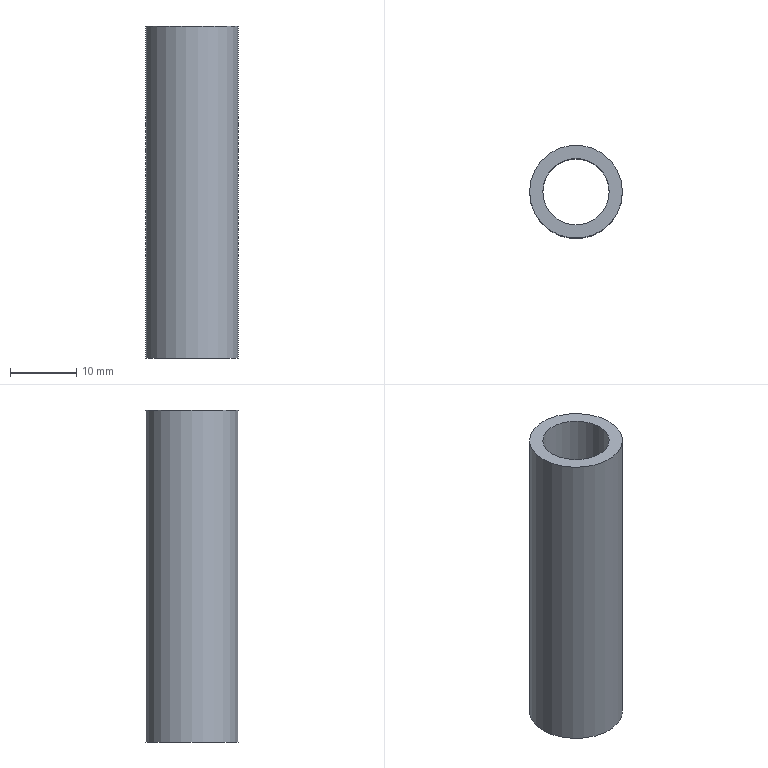Part | NX | features solid 2 | 1 solid | 4 faces | box 14 x 14 x 50 mm | volume 3770 mm3 | plane 2 | cylinder 2 | commonest cylinder face diameters 10 x1 14 x1
STEP:
#1=CARTESIAN_POINT('',(-1253.358,278.112,0.));
#2=VERTEX_POINT('',#1);
#3=CARTESIAN_POINT('',(-1258.358,278.112,0.));
#4=DIRECTION('',(0.,0.,1.));
#5=DIRECTION('',(1.,0.,0.));
#6=AXIS2_PLACEMENT_3D('',#3,#4,#5);
#7=CIRCLE('',#6,5.);
#8=EDGE_CURVE('',#2,#2,#7,.F.);
#9=ORIENTED_EDGE('',*,*,#8,.T.);
#10=EDGE_LOOP('',(#9));
#11=FACE_BOUND('',#10,.T.);
#12=CARTESIAN_POINT('',(-1265.358,278.112,0.));
#13=VERTEX_POINT('',#12);
#14=CARTESIAN_POINT('',(-1258.358,278.112,0.));
#15=DIRECTION('',(0.,0.,-1.));
#16=DIRECTION('',(-1.,0.,0.));
#17=AXIS2_PLACEMENT_3D('',#14,#15,#16);
#18=CIRCLE('',#17,7.);
#19=EDGE_CURVE('',#13,#13,#18,.T.);
#20=ORIENTED_EDGE('',*,*,#19,.F.);
#21=EDGE_LOOP('',(#20));
#22=FACE_BOUND('',#21,.T.);
#23=CARTESIAN_POINT('',(-1258.358,278.112,0.));
#24=DIRECTION('',(0.,0.,1.));
#25=DIRECTION('',(1.,0.,0.));
#26=AXIS2_PLACEMENT_3D('',#23,#24,#25);
#27=PLANE('',#26);
#28=ADVANCED_FACE('',(#11,#22),#27,.T.);
#29=CARTESIAN_POINT('',(-1253.358,278.112,-50.));
#30=VERTEX_POINT('',#29);
#31=CARTESIAN_POINT('',(-1258.358,278.112,-50.));
#32=DIRECTION('',(0.,0.,1.));
#33=DIRECTION('',(1.,0.,0.));
#34=AXIS2_PLACEMENT_3D('',#31,#32,#33);
#35=CIRCLE('',#34,5.);
#36=EDGE_CURVE('',#30,#30,#35,.F.);
#37=ORIENTED_EDGE('',*,*,#36,.F.);
#38=EDGE_LOOP('',(#37));
#39=FACE_BOUND('',#38,.T.);
#40=CARTESIAN_POINT('',(-1265.358,278.112,-50.));
#41=VERTEX_POINT('',#40);
#42=CARTESIAN_POINT('',(-1258.358,278.112,-50.));
#43=DIRECTION('',(0.,0.,-1.));
#44=DIRECTION('',(-1.,0.,0.));
#45=AXIS2_PLACEMENT_3D('',#42,#43,#44);
#46=CIRCLE('',#45,7.);
#47=EDGE_CURVE('',#41,#41,#46,.T.);
#48=ORIENTED_EDGE('',*,*,#47,.T.);
#49=EDGE_LOOP('',(#48));
#50=FACE_BOUND('',#49,.T.);
#51=CARTESIAN_POINT('',(-1258.358,278.112,-50.));
#52=DIRECTION('',(0.,0.,1.));
#53=DIRECTION('',(1.,0.,0.));
#54=AXIS2_PLACEMENT_3D('',#51,#52,#53);
#55=PLANE('',#54);
#56=ADVANCED_FACE('',(#39,#50),#55,.F.);
#57=ORIENTED_EDGE('',*,*,#8,.F.);
#58=EDGE_LOOP('',(#57));
#59=FACE_BOUND('',#58,.T.);
#60=ORIENTED_EDGE('',*,*,#36,.T.);
#61=EDGE_LOOP('',(#60));
#62=FACE_BOUND('',#61,.T.);
#63=CARTESIAN_POINT('',(-1258.358,278.112,-50.));
#64=DIRECTION('',(0.,0.,1.));
#65=DIRECTION('',(1.,0.,0.));
#66=AXIS2_PLACEMENT_3D('',#63,#64,#65);
#67=CYLINDRICAL_SURFACE('',#66,5.);
#68=ADVANCED_FACE('',(#59,#62),#67,.F.);
#69=ORIENTED_EDGE('',*,*,#19,.T.);
#70=EDGE_LOOP('',(#69));
#71=FACE_BOUND('',#70,.T.);
#72=ORIENTED_EDGE('',*,*,#47,.F.);
#73=EDGE_LOOP('',(#72));
#74=FACE_BOUND('',#73,.T.);
#75=CARTESIAN_POINT('',(-1258.358,278.112,-50.));
#76=DIRECTION('',(0.,0.,1.));
#77=DIRECTION('',(1.,0.,0.));
#78=AXIS2_PLACEMENT_3D('',#75,#76,#77);
#79=CYLINDRICAL_SURFACE('',#78,7.);
#80=ADVANCED_FACE('',(#71,#74),#79,.T.);
#81=CLOSED_SHELL('',(#28,#56,#68,#80));
#82=MANIFOLD_SOLID_BREP('',#81);
#83=(LENGTH_UNIT()NAMED_UNIT(*)SI_UNIT(.MILLI.,.METRE.));
#84=UNCERTAINTY_MEASURE_WITH_UNIT(LENGTH_MEASURE(0.00001),#83,'','');
#85=(NAMED_UNIT(*)PLANE_ANGLE_UNIT()SI_UNIT($,.RADIAN.));
#86=(NAMED_UNIT(*)SI_UNIT($,.STERADIAN.)SOLID_ANGLE_UNIT());
#87=(GEOMETRIC_REPRESENTATION_CONTEXT(3)GLOBAL_UNCERTAINTY_ASSIGNED_CONTEXT((#84))GLOBAL_UNIT_ASSIGNED_CONTEXT((#83,#85,#86))REPRESENTATION_CONTEXT('',''));
#88=ADVANCED_BREP_SHAPE_REPRESENTATION('',(#82),#87);